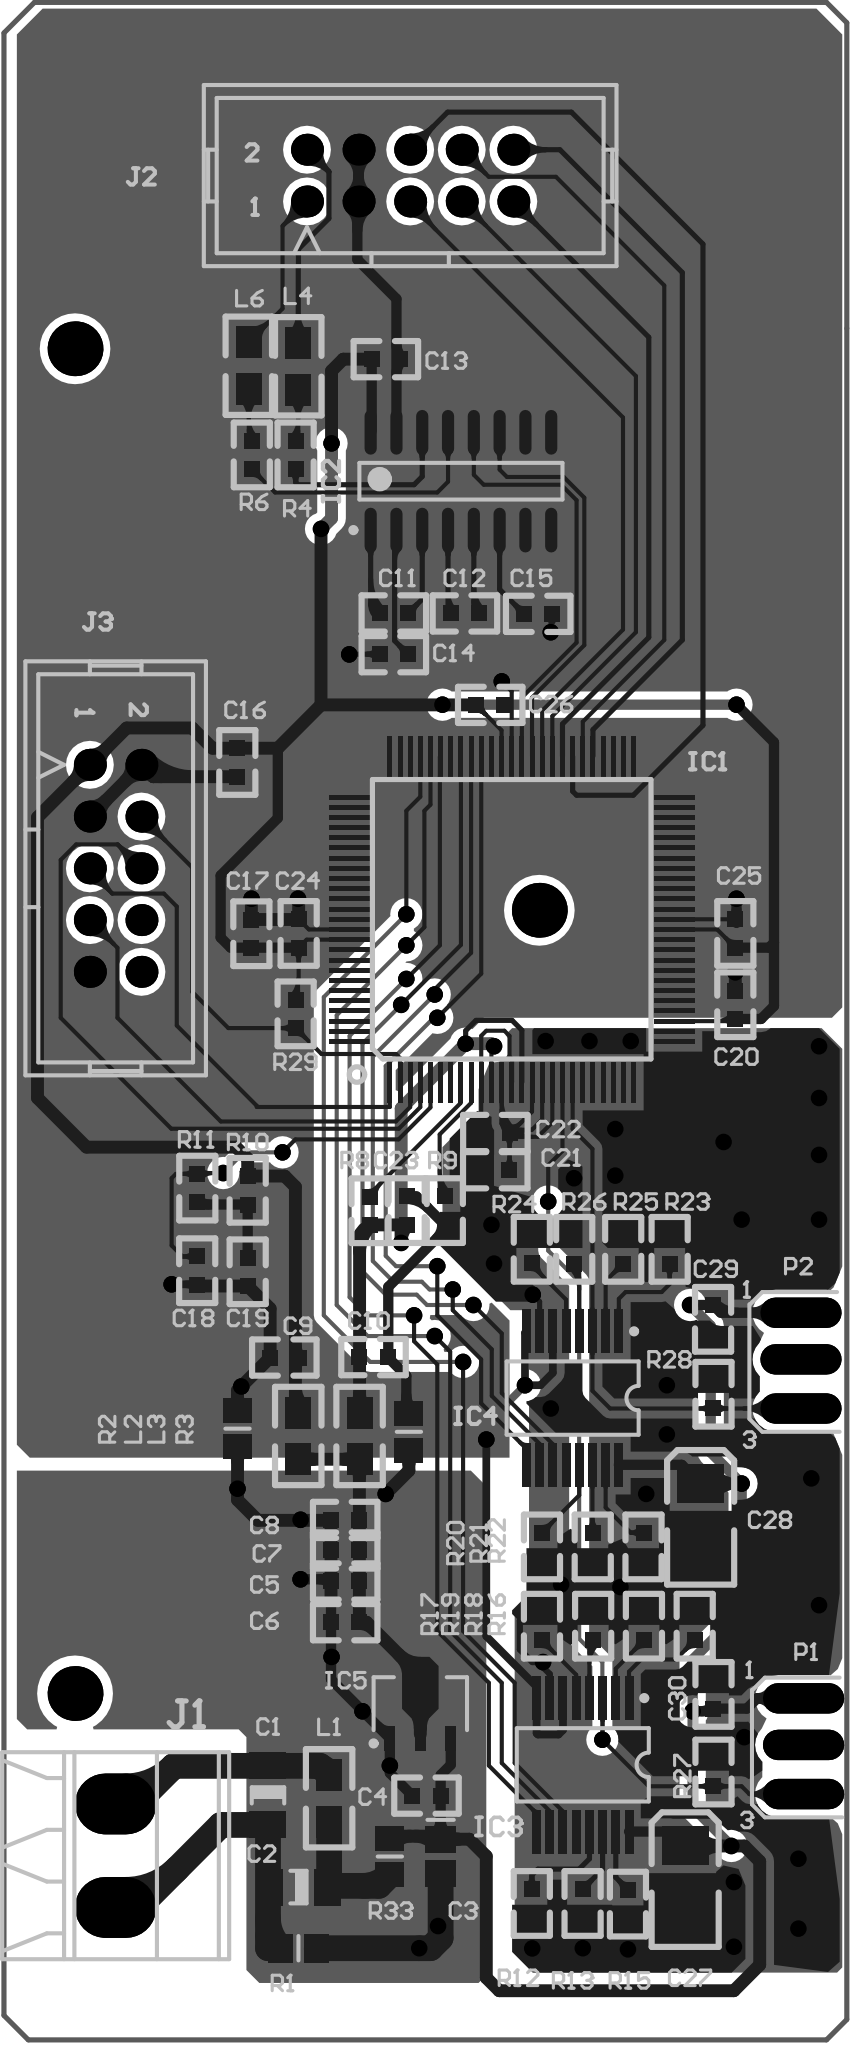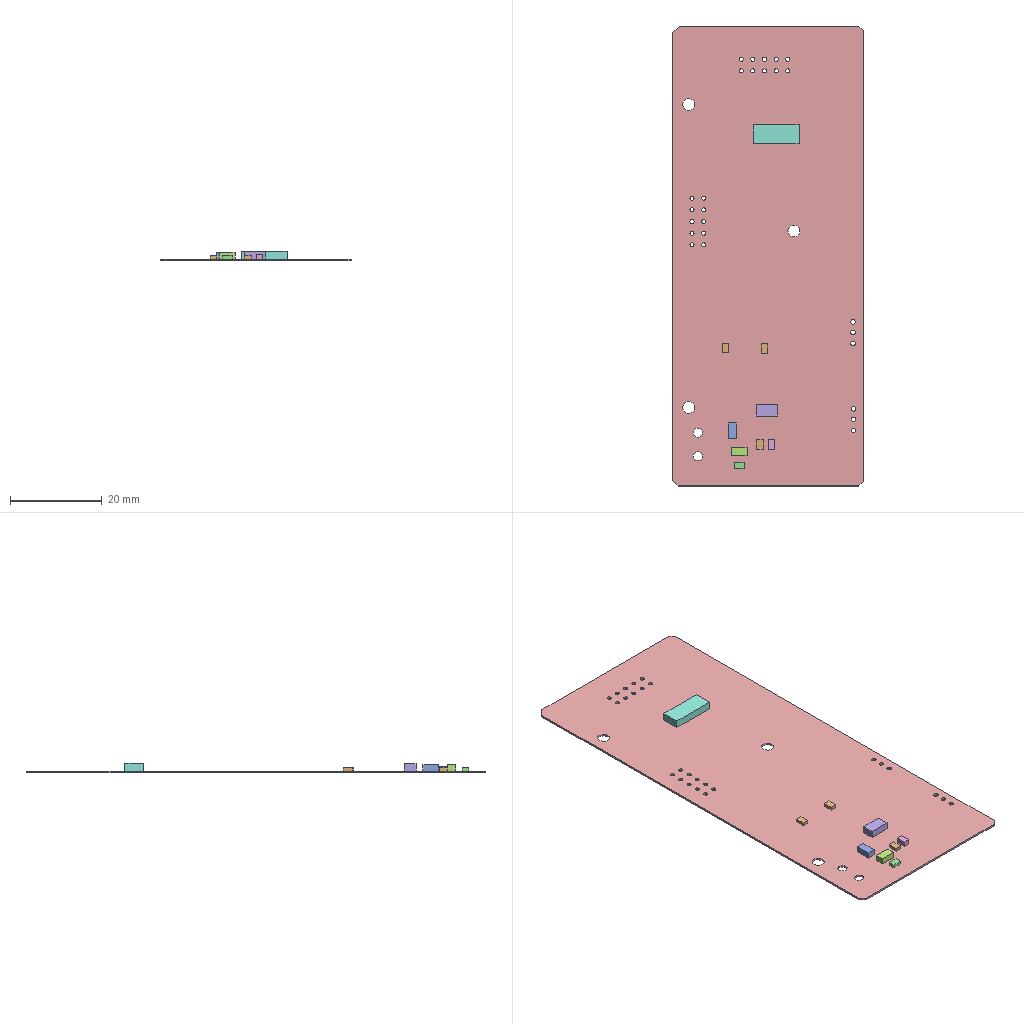Circuit board layout | Altium Designer | box 41.5 x 100 x 2.2 mm
Layer stack:
# Altium Designer layer stack of  (unit mm; dielectric type: 0 none, 1 core, 2 prepreg, 3 surface material)
index,name,kind,layer,copper_thickness_mm,dielectric_type,dielectric_thickness_mm,dielectric_material,dielectric_constant
0,TopPaste,other,,,,,,
1,TopOverlay,other,,,,,,
2,TopSolder,dielectric,,,3,0.0102,Solder Resist,3.5
3,TopLayer,copper,TopLayer,0.0356,,,,
4,Dielectric1,dielectric,,,1,0.32,FR-4,4.8
5,BottomLayer,copper,BottomLayer,0.0356,,,,
6,BottomSolder,dielectric,,,3,0.0102,Solder Resist,3.5
7,BottomOverlay,other,,,,,,
8,BottomPaste,other,,,,,,
# drill layer pairs: low layer,high layer
drill_pair,TopLayer,BottomLayer
Part placement:
Designator,Comment,Layer,Footprint,Center-X(mm),Center-Y(mm),Rotation
P1,,TopLayer,E3,39.37,14.415,0
C29,1U,TopLayer,0603,34.915,35.367,90
C30,1U,TopLayer,0603,34.935,16.957,270
P2,,TopLayer,E3,39.243,33.337,0
L6,600O/500mA-0805,TopLayer,0805,12.055,82.166,90
L4,600O/500mA-0805,TopLayer,0805,14.49,82.14,90
C1,,TopLayer,CAPC3216N,13,12,270
C27,22u,TopLayer,3528,33.54,7.803,90
J2,,TopLayer,FKV10SN,20,91.5,360
C28,22u,TopLayer,3528,34.302,25.583,90
C2,,TopLayer,CAPC3216N,14.5,7.5,180
C3,10u,TopLayer,CAPC2012N,21.5,9,270
C4,0.1U,TopLayer,0603,20.804,11.99,180
C5,100n/50V,TopLayer,0603,16.802,22.5,180
C6,10n/50V,TopLayer,0603,16.802,20.5,180
C7,0.1U,TopLayer,0603,16.802,24.02,360
C8,0.1U,TopLayer,0603,16.802,25.52,360
C9,0.1U,TopLayer,0603,13.804,33.49,180
C10,0.1U,TopLayer,0603,18.196,33.51,360
C11,100n/50V,TopLayer,0603,19.196,70.01,360
C12,100n/50V,TopLayer,0603,22.696,70.01,360
C13,100n/50V,TopLayer,0603,18.804,82.49,180
C14,100n/50V,TopLayer,0603,19.196,68.01,360
C15,100n/50V,TopLayer,0603,26.304,69.99,180
C16,0.1U,TopLayer,0603,11.49,62.696,90
C17,0.1U,TopLayer,0603,12.182,54.29,90
C18,1U,TopLayer,0603,9.515,37.751,90
C19,0.1U,TopLayer,0603,12,37.699,90
C20,0.1U,TopLayer,0603,36.01,50.804,270
C21,0.1U,TopLayer,0603,24.191,42.682,360
C22,4.7U,TopLayer,0603,24.196,44.51,360
C23,0.1U,TopLayer,0603,19.827,40.701,270
C24,0.1U,TopLayer,0603,14.51,54.304,270
C25,0.1U,TopLayer,0603,36.01,54.304,270
C26,0.1U,TopLayer,0603,23.942,65.522,180
R6,100,TopLayer,0603,12.202,77.79,270
R8,0R,TopLayer,0603,18,40.693,90
R9,0R,TopLayer,0603,21.707,40.701,90
R10,10K,TopLayer,0603,12,41.699,90
R11,1K,TopLayer,0603,9.52,41.807,90
R12,10M 1%,TopLayer,0603,25.99,6.696,90
R13,1M 1%,TopLayer,0603,28.49,6.696,90
R15,100k 1%,TopLayer,0603,30.724,6.665,90
R16,10k 1%,TopLayer,0603,34.01,20.304,270
R17,1k 1%,TopLayer,0603,26.49,20.304,90
R18,200R 1%,TopLayer,0603,31.51,20.304,270
R19,100R 1%,TopLayer,0603,29.01,20.304,270
R20,10M 1%,TopLayer,0603,26.49,24.196,90
R21,1M 1%,TopLayer,0603,28.99,24.196,90
R22,100k 1%,TopLayer,0603,31.49,24.196,90
R23,10k 1%,TopLayer,0603,32.776,38.801,270
R24,1k 1%,TopLayer,0603,25.99,38.804,90
R25,200R 1%,TopLayer,0603,30.49,38.801,270
R26,100R 1%,TopLayer,0603,28.077,38.801,270
R27,100M 1%,TopLayer,0603,34.935,13.147,270
R28,100M 1%,TopLayer,0603,34.935,31.689,270
R29,4.7K,TopLayer,0603,14.361,50.358,270
IC2,MAX3232,TopLayer,SOIC127P600-16N,22.5,76.5,90
IC4,74HC-HCT4051,TopLayer,SOIC16,28,31.5,180
R2,0R,TopLayer,6-0805_N,11.5,30,90
R3,0R,TopLayer,6-0805_N,19.939,29.845,90
L1,1UH,TopLayer,0805,16.01,11.86,270
L2,1UH,TopLayer,0805,14.49,29.64,90
L3,1UH,TopLayer,0805,17.51,29.64,270
R4,100,TopLayer,0603,14.361,77.79,270
IC3,74HC-HCT4051,TopLayer,SOIC16,28.5,13.5,180
IC5,AS117,TopLayer,SOT89L,20.5,16.05,90
R1,0R,TopLayer,6-0805_N,14.5,4.5,360
R33,0R,TopLayer,6-0805_N,19,9,90
J1,,TopLayer,MKDS3_2RMI,5.5,9.04,90
J3,,TopLayer,FKV10SN,5.5,57.5,270
Pad and via stacks:
# Altium Designer via and pad stacks of  (unit mm). Each distinct definition once, with the count of objects using it.
# via: kind,start_layer,end_layer,hole_mm,diameter_mm,mode(0 simple;1 top-mid-bottom;2 full stack),diameter_per_layer,count,example_net
# pad: kind,layer,hole_mm,hole_type(0 round;1 square;2 slot),plating,top_size,top_shape(1 round;2 rect;3 octagon;9 rounded rect),mid_size,bottom_size,mode,footprint,size_per_layer,count,example
pad,TopLayer,0,0,plated,0.762x0.762,2,0.762x0.762,0.762x0.762,0,0603,,96,C29.2
pad,TopLayer,0,0,plated,1.4x1.2,2,1.4x1.2,1.4x1.2,0,6-0805_N,,8,R2.2
pad,TopLayer,0,0,plated,0.5x1.2,2,0.5x1.2,0.5x1.2,0,SOT89L,,2,IC5.1
pad,TopLayer,0,0,plated,0.5x1.6,2,0.5x1.6,0.5x1.6,0,SOT89L,,1,IC5.2
pad,TopLayer,0,0,plated,1.8x3,3,1.8x3,1.8x3,0,SOT89L,,1,IC5.2
pad,TopLayer,0,0,plated,1.524x1.27,2,1.524x1.27,1.524x1.27,0,0805,,10,L6.1
pad,TopLayer,0,0,plated,1.905x2.286,2,1.905x2.286,1.905x2.286,0,3528,,4,C27.1
pad,TopLayer,0,0,plated,0.4x2.15,2,0.4x2.15,0.4x2.15,0,SOIC16,,32,IC4.2
pad,TopLayer,0,0,plated,1.5x1.3,2,1.5x1.3,1.5x1.3,0,CAPC2012N,,2,C3.2
pad,TopLayer,0,0,plated,1.8x1.3,2,1.8x1.3,1.8x1.3,0,CAPC3216N,,4,C1.2
pad,TopLayer,0,0,plated,0.6x2.2,1,0.6x2.2,0.6x2.2,0,SOIC127P600-16N,,16,IC2.9
pad,TopLayer,0,0,plated,2x0.23,2,2x0.23,2x0.23,0,TQFP100,,100,IC1.52
pad,MultiLayer,2.6,0,plated,2.7x2.7,1,2.7x2.7,2.7x2.7,0,,,3,0
pad,MultiLayer,1,0,plated,4x1.5,1,4x1.5,4x1.5,0,E3,,6,P1.1
pad,MultiLayer,0.889,0,plated,1.575x1.575,1,1.575x1.575,1.575x1.575,0,FKV10SN,,20,J2.6
pad,MultiLayer,2,0,plated,3x4,1,3x4,3x4,0,MKDS3_2RMI,,2,J1.2
via,TopLayer,BottomLayer,0.4064,0.8128,0,,79,GND
Copper pours:
name,layer,net,type(0 solid;1 hatched;2 none)
Mechanical 1-No Net,TopLayer,AGND_MCU,0
Mechanical 1-No Net,BottomLayer,GND,0
Mechanical 1-No Net,BottomLayer,DGND_MCU,0
Mechanical 1-No Net,BottomLayer,AGND_MCU,0
Design rules, without the lines most boards share:
# Altium Designer design rules of  (exported by Altium Designer, unit mm)
# columns: name | kind | enabled | priority | scope1 | scope2 | descriptor | typed fields (field=value)
Clearance_1 | 0 | enabled | 1 | All | InNet('DGND_MCU') | Clearance Constraint (Gap=15mil) (All),(InNet('DGND_MCU')) | gap=0.381
SilkscreenOverComponentPads | 54 | enabled | 1 | IsPad | All | Silk To Solder Mask (Clearance=10mil) (IsPad),(All) |
HoleToHoleClearance | 52 | enabled | 1 | All | All | Hole To Hole Clearance (Gap=10mil) (All),(All) | gap=0.254
DiffPairsRouting | 51 | enabled | 1 | All | All | Differential Pairs Uncoupled Length using the Gap Constraints (Min=7mil) (Max=7mil) (Prefered=7mil)  and Width Constraints (Min=15mil) (Max=15mil) (Prefered=15mil) (All) |
Testpoint | 43 | enabled | 1 | All | All | Fabrication Testpoint Style (Under Component=Yes) (All) |
TestPointUsage | 44 | enabled | 1 | All | All | Fabrication Testpoint Usage (Valid =One Required, Allow multiple per net=No) (All) |
SolderMaskExpansion | 13 | enabled | 1 | All | All | Solder Mask Expansion (Expansion =4mil) (All) | expansion=0.1016
PasteMaskExpansion | 14 | enabled | 1 | All | All | Paste Mask Expansion (Expansion =0mil) (All) | expansion=0
RoutingVias | 11 | enabled | 1 | All | All | Routing Via (MinHoleWidth=10mil) (MaxHoleWidth=28mil) (PreferredHoleWidth=10mil) (MinWidth=20mil) (MaxWidth=50mil) (PreferedWidth=20mil) (All) | via_min_hole=0.254 via_max_hole=0.7112 via_preferred_diameter=0.508 via_preferred_hole=0.254
width | 2 | enabled | 1 | All | All | Width Constraint (Min=7mil) (Max=200mil) (Preferred=8mil) (All) |
PolygonConnect | 20 | enabled | 1 | All | All | Polygon Connect Rule(Direct Connect )(Conductor Width=12mil) (Relief Angle=90 Angle) (Entries=4) (Air Gap Width=10mil) (All),(All) | connect_style(0=relief,1=direct,2=none)=1 relief_conductor_width=0.3048 relief_entries=4
PlaneClearance | 12 | enabled | 1 | All | All | Power Plane Clearance (Clearance =10mil) (All) | clearance=0.254
PlaneConnect | 6 | enabled | 1 | All | All | Power Plane Connect Rule(Direct Connect )(Expansion=20mil) (Conductor Width=10mil) (Air Gap=10mil) (Entries=4) (All) | relief_conductor_width=0.254 relief_entries=4 relief_expansion=0.508
Clearance | 0 | enabled | 2 | All | All | Clearance Constraint (Gap=8mil) (All),(All) | gap=0.2032
Classes set for this board:
# Altium Designer classes of  (member kind: 0 net, 1 component, 2 from-to, 3 pad, 4 layer, 5 differential pair, 6 design channel, 7 polygon, 8 structure, 9 xSignal)
# columns: class name | member kind | superclass | members
All From-Tos | 0 | yes |
MCU-1 | 1 | no | C1; C2; C3; C4; C5; C6; C7; C8; C9; C10; C11; C12; C13; C14; C15; C16; C17; C18; C19; C20; C21; C22; C23; C24; C25; C26; C27; C28; IC2; IC4; J2; L1; L2; L3; L4; L6; P2; R2; R3; R6; R8; R9; R10; R11; R12; R13; R15; R16; R17; R18; R19; R20; R21; R22; R23; R24; R25; R26; R27; R28; R29; IC3; IC5; R4; R1; P1; P2; R33; J1; J3; C29; C30; IC1;